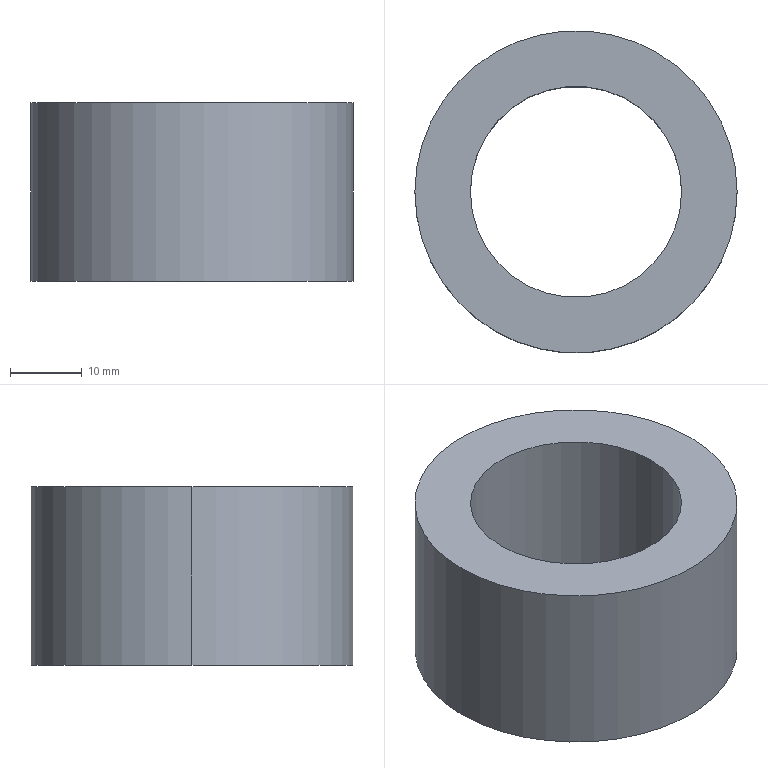Part | SolidWorks | features Extrusion 1 | 1 solid | 6 faces | box 45 x 45 x 25 mm | volume 22673 mm3 | cylinder 4 | plane 2 | commonest cylinder face diameters 29.5 x2 45 x2
STEP:
#1=CARTESIAN_POINT('',(-14.75,0.,25.));
#2=VERTEX_POINT('',#1);
#3=CARTESIAN_POINT('',(14.75,0.,25.));
#4=VERTEX_POINT('',#3);
#5=CARTESIAN_POINT('',(0.,0.,25.));
#6=DIRECTION('',(0.,0.,1.));
#7=DIRECTION('',(1.,0.,0.));
#8=AXIS2_PLACEMENT_3D('',#5,#6,#7);
#9=CIRCLE('',#8,14.75);
#10=EDGE_CURVE('',#2,#4,#9,.T.);
#11=ORIENTED_EDGE('',*,*,#10,.T.);
#12=CARTESIAN_POINT('',(14.75,0.,0.));
#13=VERTEX_POINT('',#12);
#14=CARTESIAN_POINT('',(14.75,0.,25.));
#15=DIRECTION('',(0.,0.,-1.));
#16=VECTOR('',#15,1000.);
#17=LINE('',#14,#16);
#18=EDGE_CURVE('',#4,#13,#17,.T.);
#19=ORIENTED_EDGE('',*,*,#18,.T.);
#20=CARTESIAN_POINT('',(-14.75,0.,0.));
#21=VERTEX_POINT('',#20);
#22=CARTESIAN_POINT('',(0.,0.,0.));
#23=DIRECTION('',(0.,0.,1.));
#24=DIRECTION('',(1.,0.,0.));
#25=AXIS2_PLACEMENT_3D('',#22,#23,#24);
#26=CIRCLE('',#25,14.75);
#27=EDGE_CURVE('',#21,#13,#26,.T.);
#28=ORIENTED_EDGE('',*,*,#27,.F.);
#29=CARTESIAN_POINT('',(-14.75,0.,25.));
#30=DIRECTION('',(0.,0.,-1.));
#31=VECTOR('',#30,1000.);
#32=LINE('',#29,#31);
#33=EDGE_CURVE('',#2,#21,#32,.T.);
#34=ORIENTED_EDGE('',*,*,#33,.F.);
#35=EDGE_LOOP('',(#11,#19,#28,#34));
#36=FACE_OUTER_BOUND('',#35,.T.);
#37=CARTESIAN_POINT('',(0.,0.,25.));
#38=DIRECTION('',(0.,0.,-1.));
#39=DIRECTION('',(-1.,0.,0.));
#40=AXIS2_PLACEMENT_3D('',#37,#38,#39);
#41=CYLINDRICAL_SURFACE('',#40,14.75);
#42=ADVANCED_FACE('',(#36),#41,.F.);
#43=CARTESIAN_POINT('',(22.5,0.,25.));
#44=VERTEX_POINT('',#43);
#45=CARTESIAN_POINT('',(-22.5,0.,25.));
#46=VERTEX_POINT('',#45);
#47=CARTESIAN_POINT('',(0.,0.,25.));
#48=DIRECTION('',(0.,0.,1.));
#49=DIRECTION('',(1.,0.,0.));
#50=AXIS2_PLACEMENT_3D('',#47,#48,#49);
#51=CIRCLE('',#50,22.5);
#52=EDGE_CURVE('',#44,#46,#51,.T.);
#53=ORIENTED_EDGE('',*,*,#52,.F.);
#54=CARTESIAN_POINT('',(22.5,0.,0.));
#55=VERTEX_POINT('',#54);
#56=CARTESIAN_POINT('',(22.5,0.,25.));
#57=DIRECTION('',(0.,0.,-1.));
#58=VECTOR('',#57,1000.);
#59=LINE('',#56,#58);
#60=EDGE_CURVE('',#44,#55,#59,.T.);
#61=ORIENTED_EDGE('',*,*,#60,.T.);
#62=CARTESIAN_POINT('',(-22.5,0.,0.));
#63=VERTEX_POINT('',#62);
#64=CARTESIAN_POINT('',(0.,0.,0.));
#65=DIRECTION('',(0.,0.,1.));
#66=DIRECTION('',(1.,0.,0.));
#67=AXIS2_PLACEMENT_3D('',#64,#65,#66);
#68=CIRCLE('',#67,22.5);
#69=EDGE_CURVE('',#55,#63,#68,.T.);
#70=ORIENTED_EDGE('',*,*,#69,.T.);
#71=CARTESIAN_POINT('',(-22.5,0.,25.));
#72=DIRECTION('',(0.,0.,-1.));
#73=VECTOR('',#72,1000.);
#74=LINE('',#71,#73);
#75=EDGE_CURVE('',#46,#63,#74,.T.);
#76=ORIENTED_EDGE('',*,*,#75,.F.);
#77=EDGE_LOOP('',(#53,#61,#70,#76));
#78=FACE_OUTER_BOUND('',#77,.T.);
#79=CARTESIAN_POINT('',(0.,0.,25.));
#80=DIRECTION('',(0.,0.,-1.));
#81=DIRECTION('',(-1.,0.,0.));
#82=AXIS2_PLACEMENT_3D('',#79,#80,#81);
#83=CYLINDRICAL_SURFACE('',#82,22.5);
#84=ADVANCED_FACE('',(#78),#83,.T.);
#85=CARTESIAN_POINT('',(0.,0.,25.));
#86=DIRECTION('',(0.,0.,1.));
#87=DIRECTION('',(1.,0.,0.));
#88=AXIS2_PLACEMENT_3D('',#85,#86,#87);
#89=CIRCLE('',#88,22.5);
#90=EDGE_CURVE('',#46,#44,#89,.T.);
#91=ORIENTED_EDGE('',*,*,#90,.T.);
#92=ORIENTED_EDGE('',*,*,#52,.T.);
#93=EDGE_LOOP('',(#91,#92));
#94=FACE_OUTER_BOUND('',#93,.T.);
#95=ORIENTED_EDGE('',*,*,#10,.F.);
#96=CARTESIAN_POINT('',(0.,0.,25.));
#97=DIRECTION('',(0.,0.,1.));
#98=DIRECTION('',(1.,0.,0.));
#99=AXIS2_PLACEMENT_3D('',#96,#97,#98);
#100=CIRCLE('',#99,14.75);
#101=EDGE_CURVE('',#4,#2,#100,.T.);
#102=ORIENTED_EDGE('',*,*,#101,.F.);
#103=EDGE_LOOP('',(#95,#102));
#104=FACE_BOUND('',#103,.T.);
#105=CARTESIAN_POINT('',(0.,0.,25.));
#106=DIRECTION('',(0.,0.,1.));
#107=DIRECTION('',(1.,0.,0.));
#108=AXIS2_PLACEMENT_3D('',#105,#106,#107);
#109=PLANE('',#108);
#110=ADVANCED_FACE('',(#94,#104),#109,.T.);
#111=CARTESIAN_POINT('',(0.,0.,0.));
#112=DIRECTION('',(0.,0.,1.));
#113=DIRECTION('',(1.,0.,0.));
#114=AXIS2_PLACEMENT_3D('',#111,#112,#113);
#115=CIRCLE('',#114,22.5);
#116=EDGE_CURVE('',#63,#55,#115,.T.);
#117=ORIENTED_EDGE('',*,*,#116,.F.);
#118=ORIENTED_EDGE('',*,*,#69,.F.);
#119=EDGE_LOOP('',(#117,#118));
#120=FACE_OUTER_BOUND('',#119,.T.);
#121=ORIENTED_EDGE('',*,*,#27,.T.);
#122=CARTESIAN_POINT('',(0.,0.,0.));
#123=DIRECTION('',(0.,0.,1.));
#124=DIRECTION('',(1.,0.,0.));
#125=AXIS2_PLACEMENT_3D('',#122,#123,#124);
#126=CIRCLE('',#125,14.75);
#127=EDGE_CURVE('',#13,#21,#126,.T.);
#128=ORIENTED_EDGE('',*,*,#127,.T.);
#129=EDGE_LOOP('',(#121,#128));
#130=FACE_BOUND('',#129,.T.);
#131=CARTESIAN_POINT('',(0.,0.,0.));
#132=DIRECTION('',(0.,0.,1.));
#133=DIRECTION('',(1.,0.,0.));
#134=AXIS2_PLACEMENT_3D('',#131,#132,#133);
#135=PLANE('',#134);
#136=ADVANCED_FACE('',(#120,#130),#135,.F.);
#137=ORIENTED_EDGE('',*,*,#60,.F.);
#138=ORIENTED_EDGE('',*,*,#90,.F.);
#139=ORIENTED_EDGE('',*,*,#75,.T.);
#140=ORIENTED_EDGE('',*,*,#116,.T.);
#141=EDGE_LOOP('',(#137,#138,#139,#140));
#142=FACE_OUTER_BOUND('',#141,.T.);
#143=CARTESIAN_POINT('',(0.,0.,25.));
#144=DIRECTION('',(0.,0.,-1.));
#145=DIRECTION('',(-1.,0.,0.));
#146=AXIS2_PLACEMENT_3D('',#143,#144,#145);
#147=CYLINDRICAL_SURFACE('',#146,22.5);
#148=ADVANCED_FACE('',(#142),#147,.T.);
#149=ORIENTED_EDGE('',*,*,#18,.F.);
#150=ORIENTED_EDGE('',*,*,#101,.T.);
#151=ORIENTED_EDGE('',*,*,#33,.T.);
#152=ORIENTED_EDGE('',*,*,#127,.F.);
#153=EDGE_LOOP('',(#149,#150,#151,#152));
#154=FACE_OUTER_BOUND('',#153,.T.);
#155=CARTESIAN_POINT('',(0.,0.,25.));
#156=DIRECTION('',(0.,0.,-1.));
#157=DIRECTION('',(-1.,0.,0.));
#158=AXIS2_PLACEMENT_3D('',#155,#156,#157);
#159=CYLINDRICAL_SURFACE('',#158,14.75);
#160=ADVANCED_FACE('',(#154),#159,.F.);
#161=CLOSED_SHELL('',(#42,#84,#110,#136,#148,#160));
#162=MANIFOLD_SOLID_BREP('',#161);
#163=CARTESIAN_POINT('',(0.,0.,0.));
#164=DIRECTION('',(0.,0.,1.));
#165=DIRECTION('',(1.,0.,0.));
#166=AXIS2_PLACEMENT_3D('',#163,#164,#165);
#167=(LENGTH_UNIT()NAMED_UNIT(*)SI_UNIT(.MILLI.,.METRE.));
#168=UNCERTAINTY_MEASURE_WITH_UNIT(LENGTH_MEASURE(0.00001),#167,'','');
#169=(NAMED_UNIT(*)PLANE_ANGLE_UNIT()SI_UNIT($,.RADIAN.));
#170=(NAMED_UNIT(*)SI_UNIT($,.STERADIAN.)SOLID_ANGLE_UNIT());
#171=(GEOMETRIC_REPRESENTATION_CONTEXT(3)GLOBAL_UNCERTAINTY_ASSIGNED_CONTEXT((#168))GLOBAL_UNIT_ASSIGNED_CONTEXT((#167,#169,#170))REPRESENTATION_CONTEXT('',''));
#172=ADVANCED_BREP_SHAPE_REPRESENTATION('',(#162,#166),#171);